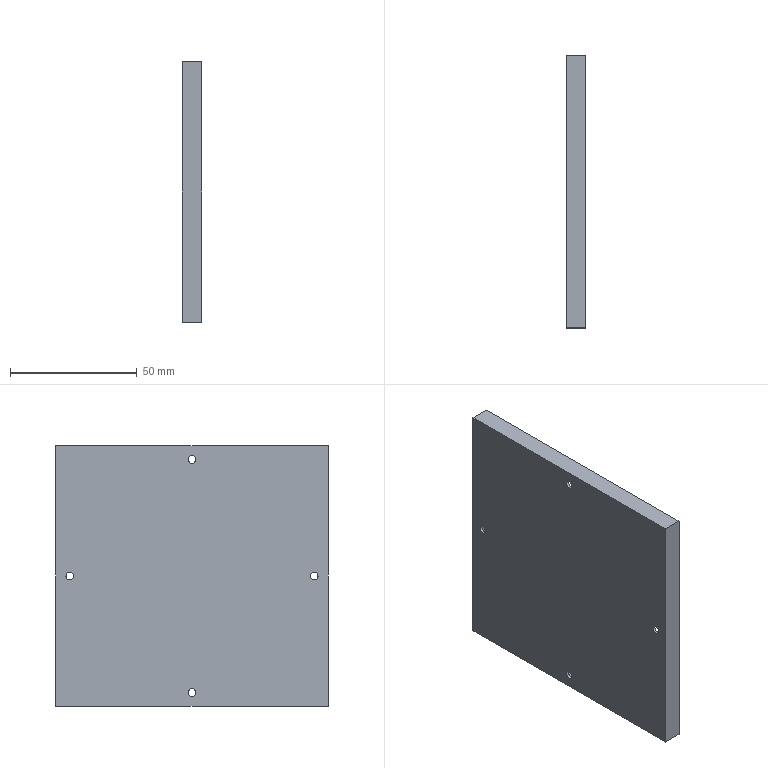Part | STEP file | 2026.6.15-Main Assembly图.sldasm-Part-136 | 1 solid | 19 faces | box 7.5 x 107.5 x 103 mm | volume 13755 mm3 | plane 11 | cylinder 8 | commonest cylinder face diameters 3 x8
STEP:
#1=CARTESIAN_POINT('',(-1736.724,609.051,4186.167));
#2=VERTEX_POINT('',#1);
#3=CARTESIAN_POINT('',(-1736.724,606.051,4186.167));
#4=VERTEX_POINT('',#3);
#5=CARTESIAN_POINT('',(-1736.724,607.551,4186.167));
#6=DIRECTION('',(-1.,0.,0.));
#7=DIRECTION('',(0.,0.,1.));
#8=AXIS2_PLACEMENT_3D('',#5,#6,#7);
#9=CIRCLE('',#8,1.5);
#10=EDGE_CURVE('',#2,#4,#9,.T.);
#11=ORIENTED_EDGE('',*,*,#10,.F.);
#12=CARTESIAN_POINT('',(-1737.724,609.051,4186.167));
#13=VERTEX_POINT('',#12);
#14=CARTESIAN_POINT('',(-1736.724,609.051,4186.167));
#15=DIRECTION('',(-1.,0.,0.));
#16=VECTOR('',#15,1000.);
#17=LINE('',#14,#16);
#18=EDGE_CURVE('',#2,#13,#17,.T.);
#19=ORIENTED_EDGE('',*,*,#18,.T.);
#20=CARTESIAN_POINT('',(-1737.724,606.051,4186.167));
#21=VERTEX_POINT('',#20);
#22=CARTESIAN_POINT('',(-1737.724,607.551,4186.167));
#23=DIRECTION('',(-1.,0.,0.));
#24=DIRECTION('',(0.,0.,1.));
#25=AXIS2_PLACEMENT_3D('',#22,#23,#24);
#26=CIRCLE('',#25,1.5);
#27=EDGE_CURVE('',#13,#21,#26,.T.);
#28=ORIENTED_EDGE('',*,*,#27,.T.);
#29=CARTESIAN_POINT('',(-1736.724,606.051,4186.167));
#30=DIRECTION('',(-1.,0.,0.));
#31=VECTOR('',#30,1000.);
#32=LINE('',#29,#31);
#33=EDGE_CURVE('',#4,#21,#32,.T.);
#34=ORIENTED_EDGE('',*,*,#33,.F.);
#35=EDGE_LOOP('',(#11,#19,#28,#34));
#36=FACE_OUTER_BOUND('',#35,.T.);
#37=CARTESIAN_POINT('',(-1736.724,607.551,4186.167));
#38=DIRECTION('',(-1.,0.,0.));
#39=DIRECTION('',(0.,-1.,0.));
#40=AXIS2_PLACEMENT_3D('',#37,#38,#39);
#41=CYLINDRICAL_SURFACE('',#40,1.5);
#42=ADVANCED_FACE('',(#36),#41,.F.);
#43=CARTESIAN_POINT('',(-1736.724,560.801,4232.167));
#44=VERTEX_POINT('',#43);
#45=CARTESIAN_POINT('',(-1736.724,557.801,4232.167));
#46=VERTEX_POINT('',#45);
#47=CARTESIAN_POINT('',(-1736.724,559.301,4232.167));
#48=DIRECTION('',(-1.,0.,0.));
#49=DIRECTION('',(0.,0.,1.));
#50=AXIS2_PLACEMENT_3D('',#47,#48,#49);
#51=CIRCLE('',#50,1.5);
#52=EDGE_CURVE('',#44,#46,#51,.T.);
#53=ORIENTED_EDGE('',*,*,#52,.F.);
#54=CARTESIAN_POINT('',(-1737.724,560.801,4232.167));
#55=VERTEX_POINT('',#54);
#56=CARTESIAN_POINT('',(-1736.724,560.801,4232.167));
#57=DIRECTION('',(-1.,0.,0.));
#58=VECTOR('',#57,1000.);
#59=LINE('',#56,#58);
#60=EDGE_CURVE('',#44,#55,#59,.T.);
#61=ORIENTED_EDGE('',*,*,#60,.T.);
#62=CARTESIAN_POINT('',(-1737.724,557.801,4232.167));
#63=VERTEX_POINT('',#62);
#64=CARTESIAN_POINT('',(-1737.724,559.301,4232.167));
#65=DIRECTION('',(-1.,0.,0.));
#66=DIRECTION('',(0.,0.,1.));
#67=AXIS2_PLACEMENT_3D('',#64,#65,#66);
#68=CIRCLE('',#67,1.5);
#69=EDGE_CURVE('',#55,#63,#68,.T.);
#70=ORIENTED_EDGE('',*,*,#69,.T.);
#71=CARTESIAN_POINT('',(-1736.724,557.801,4232.167));
#72=DIRECTION('',(-1.,0.,0.));
#73=VECTOR('',#72,1000.);
#74=LINE('',#71,#73);
#75=EDGE_CURVE('',#46,#63,#74,.T.);
#76=ORIENTED_EDGE('',*,*,#75,.F.);
#77=EDGE_LOOP('',(#53,#61,#70,#76));
#78=FACE_OUTER_BOUND('',#77,.T.);
#79=CARTESIAN_POINT('',(-1736.724,559.301,4232.167));
#80=DIRECTION('',(-1.,0.,0.));
#81=DIRECTION('',(0.,-1.,0.));
#82=AXIS2_PLACEMENT_3D('',#79,#80,#81);
#83=CYLINDRICAL_SURFACE('',#82,1.5);
#84=ADVANCED_FACE('',(#78),#83,.F.);
#85=CARTESIAN_POINT('',(-1736.724,512.551,4186.167));
#86=VERTEX_POINT('',#85);
#87=CARTESIAN_POINT('',(-1736.724,509.551,4186.167));
#88=VERTEX_POINT('',#87);
#89=CARTESIAN_POINT('',(-1736.724,511.051,4186.167));
#90=DIRECTION('',(-1.,0.,0.));
#91=DIRECTION('',(0.,0.,1.));
#92=AXIS2_PLACEMENT_3D('',#89,#90,#91);
#93=CIRCLE('',#92,1.5);
#94=EDGE_CURVE('',#86,#88,#93,.T.);
#95=ORIENTED_EDGE('',*,*,#94,.F.);
#96=CARTESIAN_POINT('',(-1737.724,512.551,4186.167));
#97=VERTEX_POINT('',#96);
#98=CARTESIAN_POINT('',(-1736.724,512.551,4186.167));
#99=DIRECTION('',(-1.,0.,0.));
#100=VECTOR('',#99,1000.);
#101=LINE('',#98,#100);
#102=EDGE_CURVE('',#86,#97,#101,.T.);
#103=ORIENTED_EDGE('',*,*,#102,.T.);
#104=CARTESIAN_POINT('',(-1737.724,509.551,4186.167));
#105=VERTEX_POINT('',#104);
#106=CARTESIAN_POINT('',(-1737.724,511.051,4186.167));
#107=DIRECTION('',(-1.,0.,0.));
#108=DIRECTION('',(0.,0.,1.));
#109=AXIS2_PLACEMENT_3D('',#106,#107,#108);
#110=CIRCLE('',#109,1.5);
#111=EDGE_CURVE('',#97,#105,#110,.T.);
#112=ORIENTED_EDGE('',*,*,#111,.T.);
#113=CARTESIAN_POINT('',(-1736.724,509.551,4186.167));
#114=DIRECTION('',(-1.,0.,0.));
#115=VECTOR('',#114,1000.);
#116=LINE('',#113,#115);
#117=EDGE_CURVE('',#88,#105,#116,.T.);
#118=ORIENTED_EDGE('',*,*,#117,.F.);
#119=EDGE_LOOP('',(#95,#103,#112,#118));
#120=FACE_OUTER_BOUND('',#119,.T.);
#121=CARTESIAN_POINT('',(-1736.724,511.051,4186.167));
#122=DIRECTION('',(-1.,0.,0.));
#123=DIRECTION('',(0.,-1.,0.));
#124=AXIS2_PLACEMENT_3D('',#121,#122,#123);
#125=CYLINDRICAL_SURFACE('',#124,1.5);
#126=ADVANCED_FACE('',(#120),#125,.F.);
#127=CARTESIAN_POINT('',(-1736.724,560.801,4140.167));
#128=VERTEX_POINT('',#127);
#129=CARTESIAN_POINT('',(-1736.724,557.801,4140.167));
#130=VERTEX_POINT('',#129);
#131=CARTESIAN_POINT('',(-1736.724,559.301,4140.167));
#132=DIRECTION('',(-1.,0.,0.));
#133=DIRECTION('',(0.,0.,1.));
#134=AXIS2_PLACEMENT_3D('',#131,#132,#133);
#135=CIRCLE('',#134,1.5);
#136=EDGE_CURVE('',#128,#130,#135,.T.);
#137=ORIENTED_EDGE('',*,*,#136,.F.);
#138=CARTESIAN_POINT('',(-1737.724,560.801,4140.167));
#139=VERTEX_POINT('',#138);
#140=CARTESIAN_POINT('',(-1736.724,560.801,4140.167));
#141=DIRECTION('',(-1.,0.,0.));
#142=VECTOR('',#141,1000.);
#143=LINE('',#140,#142);
#144=EDGE_CURVE('',#128,#139,#143,.T.);
#145=ORIENTED_EDGE('',*,*,#144,.T.);
#146=CARTESIAN_POINT('',(-1737.724,557.801,4140.167));
#147=VERTEX_POINT('',#146);
#148=CARTESIAN_POINT('',(-1737.724,559.301,4140.167));
#149=DIRECTION('',(-1.,0.,0.));
#150=DIRECTION('',(0.,0.,1.));
#151=AXIS2_PLACEMENT_3D('',#148,#149,#150);
#152=CIRCLE('',#151,1.5);
#153=EDGE_CURVE('',#139,#147,#152,.T.);
#154=ORIENTED_EDGE('',*,*,#153,.T.);
#155=CARTESIAN_POINT('',(-1736.724,557.801,4140.167));
#156=DIRECTION('',(-1.,0.,0.));
#157=VECTOR('',#156,1000.);
#158=LINE('',#155,#157);
#159=EDGE_CURVE('',#130,#147,#158,.T.);
#160=ORIENTED_EDGE('',*,*,#159,.F.);
#161=EDGE_LOOP('',(#137,#145,#154,#160));
#162=FACE_OUTER_BOUND('',#161,.T.);
#163=CARTESIAN_POINT('',(-1736.724,559.301,4140.167));
#164=DIRECTION('',(-1.,0.,0.));
#165=DIRECTION('',(0.,-1.,0.));
#166=AXIS2_PLACEMENT_3D('',#163,#164,#165);
#167=CYLINDRICAL_SURFACE('',#166,1.5);
#168=ADVANCED_FACE('',(#162),#167,.F.);
#169=CARTESIAN_POINT('',(-1737.724,505.551,4134.667));
#170=VERTEX_POINT('',#169);
#171=CARTESIAN_POINT('',(-1737.724,613.051,4134.667));
#172=VERTEX_POINT('',#171);
#173=CARTESIAN_POINT('',(-1737.724,505.551,4134.667));
#174=DIRECTION('',(0.,1.,0.));
#175=VECTOR('',#174,1000.);
#176=LINE('',#173,#175);
#177=EDGE_CURVE('',#170,#172,#176,.T.);
#178=ORIENTED_EDGE('',*,*,#177,.T.);
#179=CARTESIAN_POINT('',(-1730.224,613.051,4134.667));
#180=VERTEX_POINT('',#179);
#181=CARTESIAN_POINT('',(-1736.724,613.051,4134.667));
#182=DIRECTION('',(-1.,0.,0.));
#183=VECTOR('',#182,1000.);
#184=LINE('',#181,#183);
#185=EDGE_CURVE('',#180,#172,#184,.T.);
#186=ORIENTED_EDGE('',*,*,#185,.F.);
#187=CARTESIAN_POINT('',(-1730.224,505.551,4134.667));
#188=VERTEX_POINT('',#187);
#189=CARTESIAN_POINT('',(-1730.224,505.551,4134.667));
#190=DIRECTION('',(0.,1.,0.));
#191=VECTOR('',#190,1000.);
#192=LINE('',#189,#191);
#193=EDGE_CURVE('',#188,#180,#192,.T.);
#194=ORIENTED_EDGE('',*,*,#193,.F.);
#195=CARTESIAN_POINT('',(-1736.724,505.551,4134.667));
#196=DIRECTION('',(-1.,0.,0.));
#197=VECTOR('',#196,1000.);
#198=LINE('',#195,#197);
#199=EDGE_CURVE('',#188,#170,#198,.T.);
#200=ORIENTED_EDGE('',*,*,#199,.T.);
#201=EDGE_LOOP('',(#178,#186,#194,#200));
#202=FACE_OUTER_BOUND('',#201,.T.);
#203=CARTESIAN_POINT('',(-1736.724,505.551,4134.667));
#204=DIRECTION('',(0.,0.,1.));
#205=DIRECTION('',(0.,-1.,0.));
#206=AXIS2_PLACEMENT_3D('',#203,#204,#205);
#207=PLANE('',#206);
#208=ADVANCED_FACE('',(#202),#207,.F.);
#209=CARTESIAN_POINT('',(-1737.724,613.051,4237.667));
#210=VERTEX_POINT('',#209);
#211=CARTESIAN_POINT('',(-1737.724,613.051,4134.667));
#212=DIRECTION('',(0.,0.,1.));
#213=VECTOR('',#212,1000.);
#214=LINE('',#211,#213);
#215=EDGE_CURVE('',#172,#210,#214,.T.);
#216=ORIENTED_EDGE('',*,*,#215,.T.);
#217=CARTESIAN_POINT('',(-1730.224,613.051,4237.667));
#218=VERTEX_POINT('',#217);
#219=CARTESIAN_POINT('',(-1736.724,613.051,4237.667));
#220=DIRECTION('',(-1.,0.,0.));
#221=VECTOR('',#220,1000.);
#222=LINE('',#219,#221);
#223=EDGE_CURVE('',#218,#210,#222,.T.);
#224=ORIENTED_EDGE('',*,*,#223,.F.);
#225=CARTESIAN_POINT('',(-1730.224,613.051,4134.667));
#226=DIRECTION('',(0.,0.,1.));
#227=VECTOR('',#226,1000.);
#228=LINE('',#225,#227);
#229=EDGE_CURVE('',#180,#218,#228,.T.);
#230=ORIENTED_EDGE('',*,*,#229,.F.);
#231=ORIENTED_EDGE('',*,*,#185,.T.);
#232=EDGE_LOOP('',(#216,#224,#230,#231));
#233=FACE_OUTER_BOUND('',#232,.T.);
#234=CARTESIAN_POINT('',(-1736.724,613.051,4134.667));
#235=DIRECTION('',(0.,-1.,0.));
#236=DIRECTION('',(0.,0.,-1.));
#237=AXIS2_PLACEMENT_3D('',#234,#235,#236);
#238=PLANE('',#237);
#239=ADVANCED_FACE('',(#233),#238,.F.);
#240=CARTESIAN_POINT('',(-1737.724,505.551,4237.667));
#241=VERTEX_POINT('',#240);
#242=CARTESIAN_POINT('',(-1737.724,613.051,4237.667));
#243=DIRECTION('',(0.,-1.,0.));
#244=VECTOR('',#243,1000.);
#245=LINE('',#242,#244);
#246=EDGE_CURVE('',#210,#241,#245,.T.);
#247=ORIENTED_EDGE('',*,*,#246,.T.);
#248=CARTESIAN_POINT('',(-1730.224,505.551,4237.667));
#249=VERTEX_POINT('',#248);
#250=CARTESIAN_POINT('',(-1736.724,505.551,4237.667));
#251=DIRECTION('',(-1.,0.,0.));
#252=VECTOR('',#251,1000.);
#253=LINE('',#250,#252);
#254=EDGE_CURVE('',#249,#241,#253,.T.);
#255=ORIENTED_EDGE('',*,*,#254,.F.);
#256=CARTESIAN_POINT('',(-1730.224,613.051,4237.667));
#257=DIRECTION('',(0.,-1.,0.));
#258=VECTOR('',#257,1000.);
#259=LINE('',#256,#258);
#260=EDGE_CURVE('',#218,#249,#259,.T.);
#261=ORIENTED_EDGE('',*,*,#260,.F.);
#262=ORIENTED_EDGE('',*,*,#223,.T.);
#263=EDGE_LOOP('',(#247,#255,#261,#262));
#264=FACE_OUTER_BOUND('',#263,.T.);
#265=CARTESIAN_POINT('',(-1736.724,613.051,4237.667));
#266=DIRECTION('',(0.,0.,-1.));
#267=DIRECTION('',(0.,1.,0.));
#268=AXIS2_PLACEMENT_3D('',#265,#266,#267);
#269=PLANE('',#268);
#270=ADVANCED_FACE('',(#264),#269,.F.);
#271=ORIENTED_EDGE('',*,*,#144,.F.);
#272=CARTESIAN_POINT('',(-1736.724,559.301,4140.167));
#273=DIRECTION('',(-1.,0.,0.));
#274=DIRECTION('',(0.,0.,1.));
#275=AXIS2_PLACEMENT_3D('',#272,#273,#274);
#276=CIRCLE('',#275,1.5);
#277=EDGE_CURVE('',#130,#128,#276,.T.);
#278=ORIENTED_EDGE('',*,*,#277,.F.);
#279=ORIENTED_EDGE('',*,*,#159,.T.);
#280=CARTESIAN_POINT('',(-1737.724,559.301,4140.167));
#281=DIRECTION('',(-1.,0.,0.));
#282=DIRECTION('',(0.,0.,1.));
#283=AXIS2_PLACEMENT_3D('',#280,#281,#282);
#284=CIRCLE('',#283,1.5);
#285=EDGE_CURVE('',#147,#139,#284,.T.);
#286=ORIENTED_EDGE('',*,*,#285,.T.);
#287=EDGE_LOOP('',(#271,#278,#279,#286));
#288=FACE_OUTER_BOUND('',#287,.T.);
#289=CARTESIAN_POINT('',(-1736.724,559.301,4140.167));
#290=DIRECTION('',(-1.,0.,0.));
#291=DIRECTION('',(0.,-1.,0.));
#292=AXIS2_PLACEMENT_3D('',#289,#290,#291);
#293=CYLINDRICAL_SURFACE('',#292,1.5);
#294=ADVANCED_FACE('',(#288),#293,.F.);
#295=ORIENTED_EDGE('',*,*,#102,.F.);
#296=CARTESIAN_POINT('',(-1736.724,511.051,4186.167));
#297=DIRECTION('',(-1.,0.,0.));
#298=DIRECTION('',(0.,0.,1.));
#299=AXIS2_PLACEMENT_3D('',#296,#297,#298);
#300=CIRCLE('',#299,1.5);
#301=EDGE_CURVE('',#88,#86,#300,.T.);
#302=ORIENTED_EDGE('',*,*,#301,.F.);
#303=ORIENTED_EDGE('',*,*,#117,.T.);
#304=CARTESIAN_POINT('',(-1737.724,511.051,4186.167));
#305=DIRECTION('',(-1.,0.,0.));
#306=DIRECTION('',(0.,0.,1.));
#307=AXIS2_PLACEMENT_3D('',#304,#305,#306);
#308=CIRCLE('',#307,1.5);
#309=EDGE_CURVE('',#105,#97,#308,.T.);
#310=ORIENTED_EDGE('',*,*,#309,.T.);
#311=EDGE_LOOP('',(#295,#302,#303,#310));
#312=FACE_OUTER_BOUND('',#311,.T.);
#313=CARTESIAN_POINT('',(-1736.724,511.051,4186.167));
#314=DIRECTION('',(-1.,0.,0.));
#315=DIRECTION('',(0.,-1.,0.));
#316=AXIS2_PLACEMENT_3D('',#313,#314,#315);
#317=CYLINDRICAL_SURFACE('',#316,1.5);
#318=ADVANCED_FACE('',(#312),#317,.F.);
#319=ORIENTED_EDGE('',*,*,#60,.F.);
#320=CARTESIAN_POINT('',(-1736.724,559.301,4232.167));
#321=DIRECTION('',(-1.,0.,0.));
#322=DIRECTION('',(0.,0.,1.));
#323=AXIS2_PLACEMENT_3D('',#320,#321,#322);
#324=CIRCLE('',#323,1.5);
#325=EDGE_CURVE('',#46,#44,#324,.T.);
#326=ORIENTED_EDGE('',*,*,#325,.F.);
#327=ORIENTED_EDGE('',*,*,#75,.T.);
#328=CARTESIAN_POINT('',(-1737.724,559.301,4232.167));
#329=DIRECTION('',(-1.,0.,0.));
#330=DIRECTION('',(0.,0.,1.));
#331=AXIS2_PLACEMENT_3D('',#328,#329,#330);
#332=CIRCLE('',#331,1.5);
#333=EDGE_CURVE('',#63,#55,#332,.T.);
#334=ORIENTED_EDGE('',*,*,#333,.T.);
#335=EDGE_LOOP('',(#319,#326,#327,#334));
#336=FACE_OUTER_BOUND('',#335,.T.);
#337=CARTESIAN_POINT('',(-1736.724,559.301,4232.167));
#338=DIRECTION('',(-1.,0.,0.));
#339=DIRECTION('',(0.,-1.,0.));
#340=AXIS2_PLACEMENT_3D('',#337,#338,#339);
#341=CYLINDRICAL_SURFACE('',#340,1.5);
#342=ADVANCED_FACE('',(#336),#341,.F.);
#343=CARTESIAN_POINT('',(-1737.724,505.551,4237.667));
#344=DIRECTION('',(0.,0.,-1.));
#345=VECTOR('',#344,1000.);
#346=LINE('',#343,#345);
#347=EDGE_CURVE('',#241,#170,#346,.T.);
#348=ORIENTED_EDGE('',*,*,#347,.T.);
#349=ORIENTED_EDGE('',*,*,#199,.F.);
#350=CARTESIAN_POINT('',(-1730.224,505.551,4237.667));
#351=DIRECTION('',(0.,0.,-1.));
#352=VECTOR('',#351,1000.);
#353=LINE('',#350,#352);
#354=EDGE_CURVE('',#249,#188,#353,.T.);
#355=ORIENTED_EDGE('',*,*,#354,.F.);
#356=ORIENTED_EDGE('',*,*,#254,.T.);
#357=EDGE_LOOP('',(#348,#349,#355,#356));
#358=FACE_OUTER_BOUND('',#357,.T.);
#359=CARTESIAN_POINT('',(-1736.724,505.551,4237.667));
#360=DIRECTION('',(0.,1.,0.));
#361=DIRECTION('',(0.,0.,1.));
#362=AXIS2_PLACEMENT_3D('',#359,#360,#361);
#363=PLANE('',#362);
#364=ADVANCED_FACE('',(#358),#363,.F.);
#365=ORIENTED_EDGE('',*,*,#18,.F.);
#366=CARTESIAN_POINT('',(-1736.724,607.551,4186.167));
#367=DIRECTION('',(-1.,0.,0.));
#368=DIRECTION('',(0.,0.,1.));
#369=AXIS2_PLACEMENT_3D('',#366,#367,#368);
#370=CIRCLE('',#369,1.5);
#371=EDGE_CURVE('',#4,#2,#370,.T.);
#372=ORIENTED_EDGE('',*,*,#371,.F.);
#373=ORIENTED_EDGE('',*,*,#33,.T.);
#374=CARTESIAN_POINT('',(-1737.724,607.551,4186.167));
#375=DIRECTION('',(-1.,0.,0.));
#376=DIRECTION('',(0.,0.,1.));
#377=AXIS2_PLACEMENT_3D('',#374,#375,#376);
#378=CIRCLE('',#377,1.5);
#379=EDGE_CURVE('',#21,#13,#378,.T.);
#380=ORIENTED_EDGE('',*,*,#379,.T.);
#381=EDGE_LOOP('',(#365,#372,#373,#380));
#382=FACE_OUTER_BOUND('',#381,.T.);
#383=CARTESIAN_POINT('',(-1736.724,607.551,4186.167));
#384=DIRECTION('',(-1.,0.,0.));
#385=DIRECTION('',(0.,-1.,0.));
#386=AXIS2_PLACEMENT_3D('',#383,#384,#385);
#387=CYLINDRICAL_SURFACE('',#386,1.5);
#388=ADVANCED_FACE('',(#382),#387,.F.);
#389=CARTESIAN_POINT('',(-1736.724,612.051,4236.667));
#390=VERTEX_POINT('',#389);
#391=CARTESIAN_POINT('',(-1736.724,506.551,4236.667));
#392=VERTEX_POINT('',#391);
#393=CARTESIAN_POINT('',(-1736.724,613.051,4236.667));
#394=DIRECTION('',(0.,-1.,0.));
#395=VECTOR('',#394,1000.);
#396=LINE('',#393,#395);
#397=EDGE_CURVE('',#390,#392,#396,.T.);
#398=ORIENTED_EDGE('',*,*,#397,.T.);
#399=CARTESIAN_POINT('',(-1736.724,506.551,4135.667));
#400=VERTEX_POINT('',#399);
#401=CARTESIAN_POINT('',(-1736.724,506.551,4237.667));
#402=DIRECTION('',(0.,0.,-1.));
#403=VECTOR('',#402,1000.);
#404=LINE('',#401,#403);
#405=EDGE_CURVE('',#392,#400,#404,.T.);
#406=ORIENTED_EDGE('',*,*,#405,.T.);
#407=CARTESIAN_POINT('',(-1736.724,612.051,4135.667));
#408=VERTEX_POINT('',#407);
#409=CARTESIAN_POINT('',(-1736.724,505.551,4135.667));
#410=DIRECTION('',(0.,1.,0.));
#411=VECTOR('',#410,1000.);
#412=LINE('',#409,#411);
#413=EDGE_CURVE('',#400,#408,#412,.T.);
#414=ORIENTED_EDGE('',*,*,#413,.T.);
#415=CARTESIAN_POINT('',(-1736.724,612.051,4134.667));
#416=DIRECTION('',(0.,0.,1.));
#417=VECTOR('',#416,1000.);
#418=LINE('',#415,#417);
#419=EDGE_CURVE('',#408,#390,#418,.T.);
#420=ORIENTED_EDGE('',*,*,#419,.T.);
#421=EDGE_LOOP('',(#398,#406,#414,#420));
#422=FACE_OUTER_BOUND('',#421,.T.);
#423=ORIENTED_EDGE('',*,*,#325,.T.);
#424=ORIENTED_EDGE('',*,*,#52,.T.);
#425=EDGE_LOOP('',(#423,#424));
#426=FACE_BOUND('',#425,.T.);
#427=ORIENTED_EDGE('',*,*,#301,.T.);
#428=ORIENTED_EDGE('',*,*,#94,.T.);
#429=EDGE_LOOP('',(#427,#428));
#430=FACE_BOUND('',#429,.T.);
#431=ORIENTED_EDGE('',*,*,#277,.T.);
#432=ORIENTED_EDGE('',*,*,#136,.T.);
#433=EDGE_LOOP('',(#431,#432));
#434=FACE_BOUND('',#433,.T.);
#435=ORIENTED_EDGE('',*,*,#371,.T.);
#436=ORIENTED_EDGE('',*,*,#10,.T.);
#437=EDGE_LOOP('',(#435,#436));
#438=FACE_BOUND('',#437,.T.);
#439=CARTESIAN_POINT('',(-1736.724,559.301,4232.167));
#440=DIRECTION('',(-1.,0.,0.));
#441=DIRECTION('',(0.,-1.,0.));
#442=AXIS2_PLACEMENT_3D('',#439,#440,#441);
#443=PLANE('',#442);
#444=ADVANCED_FACE('',(#422,#426,#430,#434,#438),#443,.F.);
#445=ORIENTED_EDGE('',*,*,#177,.F.);
#446=ORIENTED_EDGE('',*,*,#347,.F.);
#447=ORIENTED_EDGE('',*,*,#246,.F.);
#448=ORIENTED_EDGE('',*,*,#215,.F.);
#449=EDGE_LOOP('',(#445,#446,#447,#448));
#450=FACE_OUTER_BOUND('',#449,.T.);
#451=ORIENTED_EDGE('',*,*,#333,.F.);
#452=ORIENTED_EDGE('',*,*,#69,.F.);
#453=EDGE_LOOP('',(#451,#452));
#454=FACE_BOUND('',#453,.T.);
#455=ORIENTED_EDGE('',*,*,#309,.F.);
#456=ORIENTED_EDGE('',*,*,#111,.F.);
#457=EDGE_LOOP('',(#455,#456));
#458=FACE_BOUND('',#457,.T.);
#459=ORIENTED_EDGE('',*,*,#285,.F.);
#460=ORIENTED_EDGE('',*,*,#153,.F.);
#461=EDGE_LOOP('',(#459,#460));
#462=FACE_BOUND('',#461,.T.);
#463=ORIENTED_EDGE('',*,*,#379,.F.);
#464=ORIENTED_EDGE('',*,*,#27,.F.);
#465=EDGE_LOOP('',(#463,#464));
#466=FACE_BOUND('',#465,.T.);
#467=CARTESIAN_POINT('',(-1737.724,559.301,4232.167));
#468=DIRECTION('',(-1.,0.,0.));
#469=DIRECTION('',(0.,-1.,0.));
#470=AXIS2_PLACEMENT_3D('',#467,#468,#469);
#471=PLANE('',#470);
#472=ADVANCED_FACE('',(#450,#454,#458,#462,#466),#471,.T.);
#473=CARTESIAN_POINT('',(-1730.224,506.551,4236.667));
#474=VERTEX_POINT('',#473);
#475=CARTESIAN_POINT('',(-1730.224,506.551,4135.667));
#476=VERTEX_POINT('',#475);
#477=CARTESIAN_POINT('',(-1730.224,506.551,4237.667));
#478=DIRECTION('',(0.,0.,-1.));
#479=VECTOR('',#478,1000.);
#480=LINE('',#477,#479);
#481=EDGE_CURVE('',#474,#476,#480,.T.);
#482=ORIENTED_EDGE('',*,*,#481,.F.);
#483=CARTESIAN_POINT('',(-1730.224,612.051,4236.667));
#484=VERTEX_POINT('',#483);
#485=CARTESIAN_POINT('',(-1730.224,613.051,4236.667));
#486=DIRECTION('',(0.,-1.,0.));
#487=VECTOR('',#486,1000.);
#488=LINE('',#485,#487);
#489=EDGE_CURVE('',#484,#474,#488,.T.);
#490=ORIENTED_EDGE('',*,*,#489,.F.);
#491=CARTESIAN_POINT('',(-1730.224,612.051,4135.667));
#492=VERTEX_POINT('',#491);
#493=CARTESIAN_POINT('',(-1730.224,612.051,4134.667));
#494=DIRECTION('',(0.,0.,1.));
#495=VECTOR('',#494,1000.);
#496=LINE('',#493,#495);
#497=EDGE_CURVE('',#492,#484,#496,.T.);
#498=ORIENTED_EDGE('',*,*,#497,.F.);
#499=CARTESIAN_POINT('',(-1730.224,505.551,4135.667));
#500=DIRECTION('',(0.,1.,0.));
#501=VECTOR('',#500,1000.);
#502=LINE('',#499,#501);
#503=EDGE_CURVE('',#476,#492,#502,.T.);
#504=ORIENTED_EDGE('',*,*,#503,.F.);
#505=EDGE_LOOP('',(#482,#490,#498,#504));
#506=FACE_BOUND('',#505,.T.);
#507=ORIENTED_EDGE('',*,*,#260,.T.);
#508=ORIENTED_EDGE('',*,*,#354,.T.);
#509=ORIENTED_EDGE('',*,*,#193,.T.);
#510=ORIENTED_EDGE('',*,*,#229,.T.);
#511=EDGE_LOOP('',(#507,#508,#509,#510));
#512=FACE_OUTER_BOUND('',#511,.T.);
#513=CARTESIAN_POINT('',(-1730.224,613.051,4237.667));
#514=DIRECTION('',(-1.,0.,0.));
#515=DIRECTION('',(0.,-1.,0.));
#516=AXIS2_PLACEMENT_3D('',#513,#514,#515);
#517=PLANE('',#516);
#518=ADVANCED_FACE('',(#506,#512),#517,.F.);
#519=ORIENTED_EDGE('',*,*,#481,.T.);
#520=CARTESIAN_POINT('',(-1736.724,506.551,4135.667));
#521=DIRECTION('',(1.,0.,0.));
#522=VECTOR('',#521,1000.);
#523=LINE('',#520,#522);
#524=EDGE_CURVE('',#400,#476,#523,.T.);
#525=ORIENTED_EDGE('',*,*,#524,.F.);
#526=ORIENTED_EDGE('',*,*,#405,.F.);
#527=CARTESIAN_POINT('',(-1736.724,506.551,4236.667));
#528=DIRECTION('',(1.,0.,0.));
#529=VECTOR('',#528,1000.);
#530=LINE('',#527,#529);
#531=EDGE_CURVE('',#392,#474,#530,.T.);
#532=ORIENTED_EDGE('',*,*,#531,.T.);
#533=EDGE_LOOP('',(#519,#525,#526,#532));
#534=FACE_OUTER_BOUND('',#533,.T.);
#535=CARTESIAN_POINT('',(-1736.724,506.551,4237.667));
#536=DIRECTION('',(0.,-1.,0.));
#537=DIRECTION('',(0.,0.,-1.));
#538=AXIS2_PLACEMENT_3D('',#535,#536,#537);
#539=PLANE('',#538);
#540=ADVANCED_FACE('',(#534),#539,.F.);
#541=ORIENTED_EDGE('',*,*,#503,.T.);
#542=CARTESIAN_POINT('',(-1736.724,612.051,4135.667));
#543=DIRECTION('',(1.,0.,0.));
#544=VECTOR('',#543,1000.);
#545=LINE('',#542,#544);
#546=EDGE_CURVE('',#408,#492,#545,.T.);
#547=ORIENTED_EDGE('',*,*,#546,.F.);
#548=ORIENTED_EDGE('',*,*,#413,.F.);
#549=ORIENTED_EDGE('',*,*,#524,.T.);
#550=EDGE_LOOP('',(#541,#547,#548,#549));
#551=FACE_OUTER_BOUND('',#550,.T.);
#552=CARTESIAN_POINT('',(-1736.724,505.551,4135.667));
#553=DIRECTION('',(0.,0.,-1.));
#554=DIRECTION('',(0.,1.,0.));
#555=AXIS2_PLACEMENT_3D('',#552,#553,#554);
#556=PLANE('',#555);
#557=ADVANCED_FACE('',(#551),#556,.F.);
#558=ORIENTED_EDGE('',*,*,#497,.T.);
#559=CARTESIAN_POINT('',(-1736.724,612.051,4236.667));
#560=DIRECTION('',(1.,0.,0.));
#561=VECTOR('',#560,1000.);
#562=LINE('',#559,#561);
#563=EDGE_CURVE('',#390,#484,#562,.T.);
#564=ORIENTED_EDGE('',*,*,#563,.F.);
#565=ORIENTED_EDGE('',*,*,#419,.F.);
#566=ORIENTED_EDGE('',*,*,#546,.T.);
#567=EDGE_LOOP('',(#558,#564,#565,#566));
#568=FACE_OUTER_BOUND('',#567,.T.);
#569=CARTESIAN_POINT('',(-1736.724,612.051,4134.667));
#570=DIRECTION('',(0.,1.,0.));
#571=DIRECTION('',(0.,0.,1.));
#572=AXIS2_PLACEMENT_3D('',#569,#570,#571);
#573=PLANE('',#572);
#574=ADVANCED_FACE('',(#568),#573,.F.);
#575=ORIENTED_EDGE('',*,*,#489,.T.);
#576=ORIENTED_EDGE('',*,*,#531,.F.);
#577=ORIENTED_EDGE('',*,*,#397,.F.);
#578=ORIENTED_EDGE('',*,*,#563,.T.);
#579=EDGE_LOOP('',(#575,#576,#577,#578));
#580=FACE_OUTER_BOUND('',#579,.T.);
#581=CARTESIAN_POINT('',(-1736.724,613.051,4236.667));
#582=DIRECTION('',(0.,0.,1.));
#583=DIRECTION('',(0.,-1.,0.));
#584=AXIS2_PLACEMENT_3D('',#581,#582,#583);
#585=PLANE('',#584);
#586=ADVANCED_FACE('',(#580),#585,.F.);
#587=CLOSED_SHELL('',(#42,#84,#126,#168,#208,#239,#270,#294,#318,#342,#364,#388,#444,#472,#518,#540,#557,#574,#586));
#588=MANIFOLD_SOLID_BREP('',#587);
#589=CARTESIAN_POINT('',(0.,0.,0.));
#590=DIRECTION('',(0.,0.,1.));
#591=DIRECTION('',(1.,0.,0.));
#592=AXIS2_PLACEMENT_3D('',#589,#590,#591);
#593=(LENGTH_UNIT()NAMED_UNIT(*)SI_UNIT(.MILLI.,.METRE.));
#594=UNCERTAINTY_MEASURE_WITH_UNIT(LENGTH_MEASURE(0.00001),#593,'','');
#595=(NAMED_UNIT(*)PLANE_ANGLE_UNIT()SI_UNIT($,.RADIAN.));
#596=(NAMED_UNIT(*)SI_UNIT($,.STERADIAN.)SOLID_ANGLE_UNIT());
#597=(GEOMETRIC_REPRESENTATION_CONTEXT(3)GLOBAL_UNCERTAINTY_ASSIGNED_CONTEXT((#594))GLOBAL_UNIT_ASSIGNED_CONTEXT((#593,#595,#596))REPRESENTATION_CONTEXT('',''));
#598=ADVANCED_BREP_SHAPE_REPRESENTATION('',(#588,#592),#597);